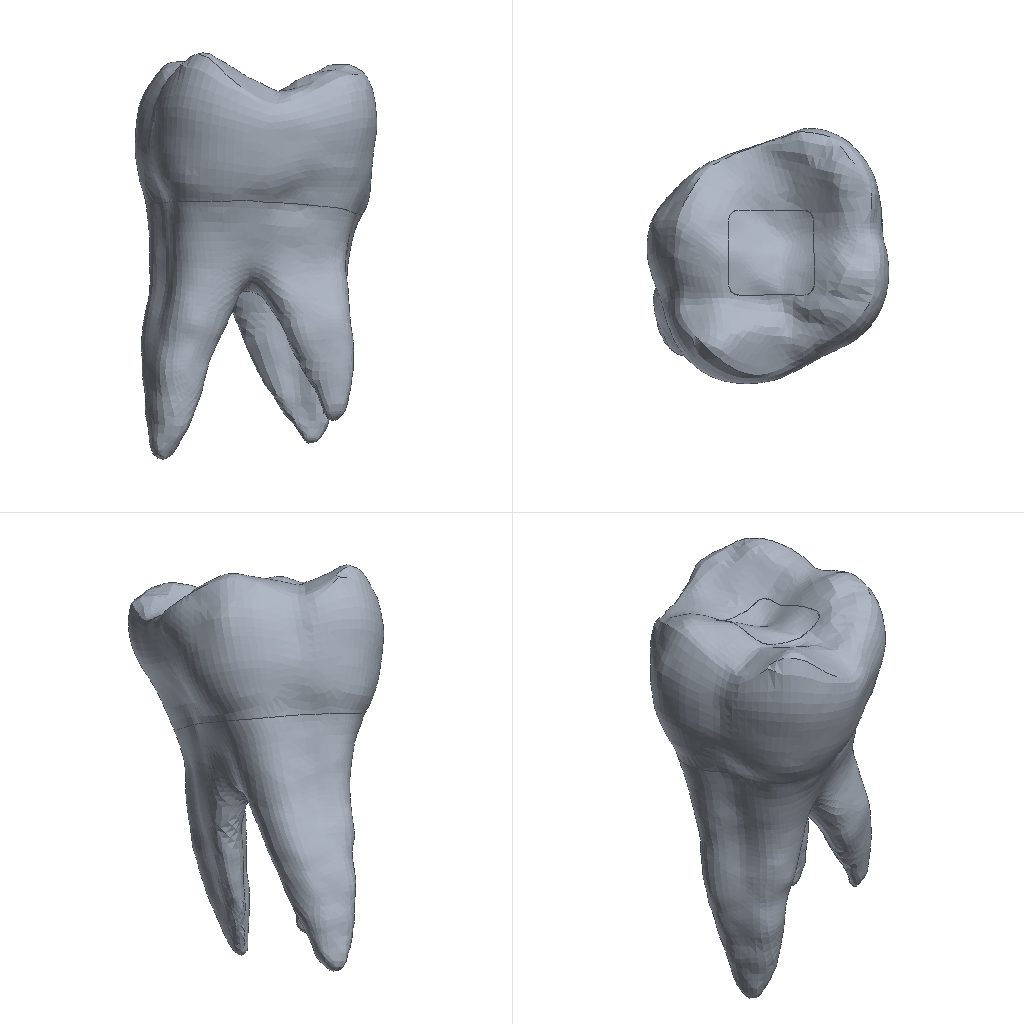Simulation study | abaqus
Set-up summary:
category,name,step,type,value,unit,region
solver,abaqus
solver,version,,,Abaqus/Standard 2020
units,not stated in the deck,,not stated
analysis,deck,,thermal,thermal
load_step,Step-1,Step-1,thermal
load_step,requested,,,1
mesh,nodes,,,60960
mesh,elements,,,308773
element_type,DC3D4,,solid,308773
load,load commands in deck,,count,3
bc,support commands in deck,,count,1
material,DENTIN,,in results
material,ENAMEL,,in results
material,PULP,,in results
material,REIN,,in results
check,setup vs results,,match,"per instance, exact: element labels, types and connectivity; labels of the nodes the elements use; coordinates of those nodes at SINGLE_PRECISION in 4 of 4 instance(s)"
Abaqus input file, long lists of numbers shortened:
*Heading
** Job name: Job-1 Model name: TRY-15
** Generated by: Abaqus/CAE 2020
*Preprint, echo=NO, model=NO, history=NO, contact=NO
**
** PARTS
**
*Part, name=DETIN
*Node
      1,  -35.692,   -2.365,   11.829
      2,    -35.895,  -2.58,   11.818
** (44272 more lines like these left out)
*Element, type=DC3D4
     1, 12572, 12573, 12574, 12575
     2, 12572, 12576, 12577, 12578
** (231746 more lines like these left out)
*Nset, nset=DENTIN, generate
     1,  44274,      1
*Elset, elset=DENTIN, generate
      1,  231748,       1
*Elset, elset=_D-E_S3, internal
     66,    221,    538,    591,   1106,   2340,   3456,   4665,   4825,   4830,   5177,   6829,   6834,   7005,   7707,   8070
   8084,   8158,   8403,  10011,  10111,  10508,  10907,  10925,  12002,  12020,  12028,  12047,  12055,  12064,  12070,  12081
** (190 more lines like these left out)
*Elset, elset=_D-E_S4, internal
   1151,   1255,   1465,   1975,   5425,   6041,   7050,   8616,   8690,  10700,  10803,  11765,  13500,  15389,  15707,  23011
  25378,  25675,  25833,  25975,  26199,  26378,  29076,  29227,  29399,  29698,  30054,  30055,  32651,  33230,  33251,  33540
** (14 more lines like these left out)
*Elset, elset=_D-E_S2, internal
   1416,   1904,   2071,   4147,   5318,   7713,   9028,  10010,  10024,  10486,  12316,  12331,  12948,  13747,  22977,  25703
  25749,  25763,  25879,  25990,  26349,  29128,  29407,  29462,  29466,  29473,  29507,  29584,  29591,  29596,  29602,  29663
** (15 more lines like these left out)
*Elset, elset=_D-E_S1, internal
   5733,  11885,  12062,  12813,  13750,  13996,  14000,  14123,  14282,  14419,  24990,  25641,  25720,  25947,  25990,  26290
  26311,  27827,  29314,  29569,  29677,  29698,  30069,  30103,  32924,  33012,  33024,  33156,  33187,  33225,  33251,  33472
** (14 more lines like these left out)
*Elset, elset=_D-R_S3, internal
   5734,   6686,   6964,   7429,   7457,   9157,  10041,  10109,  10355,  11055,  12136,  12138,  12290,  12337,  12498,  12806
  12815,  12836,  12952,  13340,  13438,  13445,  13514,  13552,  13755,  13855,  13946,  14031,  14061,  14116,  14465,  20872
** (34 more lines like these left out)
*Elset, elset=_D-R_S4, internal
   6450,  25895,  29323,  29359,  30035,  32601,  33024,  36247,  46250,  49133,  97027,  99941, 107238, 112465, 121080, 131481
 133725, 137569, 139854, 142716, 144027, 164053, 170285, 176348, 189297, 221559
*Elset, elset=_D-R_S1, internal
  22984,  25706,  25921,  26205,  29095,  29096,  29821,  32855,  32937,  36596,  38121,  40083,  43461,  85559,  87495,  87596
 103786, 108863, 111221, 111935, 142008, 143946, 149051, 149554, 162747, 167614, 169637, 175206, 179761, 183881, 205859
*Elset, elset=_D-R_S2, internal
   4550,   6181,  11968,  22962,  22985,  23017,  25463,  25798,  25843,  26000,  26085,  26148,  26231,  29060,  29073,  29092
  29104,  29110,  29251,  29725,  29755,  29846,  32441,  32442,  32829,  32854,  32886,  32936,  33212, 138750
*Elset, elset=_D-P_S3, internal
     38,    157,    343,    405,    497,    643,    734,    945,   1441,   1678,   1894,   2442,   2647,   2918,   2976,   3287
   3440,   3483,   3969,   3999,   4509,   4512,   4551,   4620,   4641,   5890,   6421,   6490,   6691,   6812,   7019,   7151
** (652 more lines like these left out)
*Elset, elset=_D-P_S2, internal
    529,    944,    949,   1000,   1007,   1584,   1585,   1731,   4072,   4205,   4418,   5149,   5374,   5549,   6425,   7188
   7376,   7666,   8660,   9682,   9846,   9975,  10014,  10029,  10033,  10837,  10842,  13021,  13267,  13346,  13366,  13528
** (37 more lines like these left out)
*Elset, elset=_D-P_S4, internal
    426,    464,   1062,   1239,   1483,   1662,   2900,   4324,   4745,   4791,   4969,   5155,   5215,   5630,   6037,   6276
   6317,   6334,   6460,   6528,   6608,   6650,   7446,   7587,   7627,   8168,   9240,   9388,   9636,   9662,   9764,   9791
** (58 more lines like these left out)
*Elset, elset=_D-P_S1, internal
   1399,   4556,  12933,  13162,  13300,  13832,  14011,  14304,  14360,  14492,  15342,  16105,  16819,  16854,  17440,  18440
  18786,  18988,  19585,  19938,  19957,  19982,  19987,  21704,  21817,  22118,  22288,  23956,  24055,  24170,  24432,  27384
** (47 more lines like these left out)
*Elset, elset=_D-E_S3_1, internal
     66,    221,    538,    591,   1106,   2340,   3456,   4665,   4825,   4830,   5177,   6829,   6834,   7005,   7707,   8070
   8084,   8158,   8403,  10011,  10111,  10508,  10907,  10925,  12002,  12020,  12028,  12047,  12055,  12064,  12070,  12081
** (190 more lines like these left out)
*Elset, elset=_D-E_S4_1, internal
   1151,   1255,   1465,   1975,   5425,   6041,   7050,   8616,   8690,  10700,  10803,  11765,  13500,  15389,  15707,  23011
  25378,  25675,  25833,  25975,  26199,  26378,  29076,  29227,  29399,  29698,  30054,  30055,  32651,  33230,  33251,  33540
** (14 more lines like these left out)
*Elset, elset=_D-E_S2_1, internal
   1416,   1904,   2071,   4147,   5318,   7713,   9028,  10010,  10024,  10486,  12316,  12331,  12948,  13747,  22977,  25703
  25749,  25763,  25879,  25990,  26349,  29128,  29407,  29462,  29466,  29473,  29507,  29584,  29591,  29596,  29602,  29663
** (15 more lines like these left out)
*Elset, elset=_D-E_S1_1, internal
   5733,  11885,  12062,  12813,  13750,  13996,  14000,  14123,  14282,  14419,  24990,  25641,  25720,  25947,  25990,  26290
  26311,  27827,  29314,  29569,  29677,  29698,  30069,  30103,  32924,  33012,  33024,  33156,  33187,  33225,  33251,  33472
** (14 more lines like these left out)
*Surface, type=ELEMENT, name=D-E
_D-E_S3_1, S3
_D-E_S4_1, S4
_D-E_S2_1, S2
_D-E_S1_1, S1
*Elset, elset=_D-R_S3_1, internal
   5734,   6686,   6964,   7429,   7457,   9157,  10041,  10109,  10355,  11055,  12136,  12138,  12290,  12337,  12498,  12806
  12815,  12836,  12952,  13340,  13438,  13445,  13514,  13552,  13755,  13855,  13946,  14031,  14061,  14116,  14465,  20872
** (34 more lines like these left out)
*Elset, elset=_D-R_S4_1, internal
   6450,  25895,  29323,  29359,  30035,  32601,  33024,  36247,  46250,  49133,  97027,  99941, 107238, 112465, 121080, 131481
 133725, 137569, 139854, 142716, 144027, 164053, 170285, 176348, 189297, 221559
*Elset, elset=_D-R_S2_1, internal
   4550,   6181,  11968,  22962,  22985,  23017,  25463,  25798,  25843,  26000,  26085,  26148,  26231,  29060,  29073,  29092
  29104,  29110,  29251,  29725,  29755,  29846,  32441,  32442,  32829,  32854,  32886,  32936,  33212, 138750
*Elset, elset=_D-R_S1_1, internal
  22984,  25706,  25921,  26205,  29095,  29096,  29821,  32855,  32937,  36596,  38121,  40083,  43461,  85559,  87495,  87596
 103786, 108863, 111221, 111935, 142008, 143946, 149051, 149554, 162747, 167614, 169637, 175206, 179761, 183881, 205859
*Surface, type=ELEMENT, name=D-R
_D-R_S3_1, S3
_D-R_S4_1, S4
_D-R_S2_1, S2
_D-R_S1_1, S1
*Elset, elset=_D-P_S3_1, internal
     38,    157,    343,    405,    497,    643,    734,    945,   1441,   1678,   1894,   2442,   2647,   2918,   2976,   3287
   3440,   3483,   3969,   3999,   4509,   4512,   4551,   4620,   4641,   5890,   6421,   6490,   6691,   6812,   7019,   7151
** (652 more lines like these left out)
*Elset, elset=_D-P_S2_1, internal
    529,    944,    949,   1000,   1007,   1584,   1585,   1731,   4072,   4205,   4418,   5149,   5374,   5549,   6425,   7188
   7376,   7666,   8660,   9682,   9846,   9975,  10014,  10029,  10033,  10837,  10842,  13021,  13267,  13346,  13366,  13528
** (37 more lines like these left out)
*Elset, elset=_D-P_S4_1, internal
    426,    464,   1062,   1239,   1483,   1662,   2900,   4324,   4745,   4791,   4969,   5155,   5215,   5630,   6037,   6276
   6317,   6334,   6460,   6528,   6608,   6650,   7446,   7587,   7627,   8168,   9240,   9388,   9636,   9662,   9764,   9791
** (58 more lines like these left out)
*Elset, elset=_D-P_S1_1, internal
   1399,   4556,  12933,  13162,  13300,  13832,  14011,  14304,  14360,  14492,  15342,  16105,  16819,  16854,  17440,  18440
  18786,  18988,  19585,  19938,  19957,  19982,  19987,  21704,  21817,  22118,  22288,  23956,  24055,  24170,  24432,  27384
** (47 more lines like these left out)
*Surface, type=ELEMENT, name=D-P
_D-P_S3_1, S3
_D-P_S2_1, S2
_D-P_S4_1, S4
_D-P_S1_1, S1
** Section: Section-1-DENTIN
*Solid Section, elset=DENTIN, material=DENTIN
,
*End Part
**
*Part, name=ENAMEL
*Node
      1,  -28.183,   3.777,   29.443
      2,  -28.797,   3.864,   29.053
** (5959 more lines like these left out)
*Element, type=DC3D4
    1, 3366, 3367, 3368, 3114
    2, 3369, 3370, 3371, 3372
** (25664 more lines like these left out)
*Nset, nset=ENAMEL, generate
    1,  5961,     1
*Elset, elset=ENAMEL, generate
     1,  25666,      1
*Elset, elset=_E-D_S1, internal
   115,   143,   670,   914,   964,  1200,  1350,  1379,  1460,  1844,  1861,  2247,  2711,  2858,  2866,  3191
  3271,  3777,  3821,  4171,  4200,  4408,  4537,  4602,  4740,  5040,  5071,  5085,  5183,  5429,  5746,  5921
** (12 more lines like these left out)
*Elset, elset=_E-D_S4, internal
   165,   209,   333,   368,   447,   459,   496,   499,   610,   631,   750,   824,   855,   876,   902,   978
   983,  1041,  1208,  1213,  1267,  1312,  1410,  1616,  1861,  1869,  1872,  1965,  2087,  2269,  2291,  2336
** (16 more lines like these left out)
*Elset, elset=_E-D_S3, internal
   133,   211,   581,   754,  1159,  1191,  1305,  1938,  1941,  2050,  2127,  2135,  2196,  2208,  2236,  2586
  2716,  2832,  3492,  3610,  3621,  3742,  3795,  3878,  3928,  4050,  4080,  4109,  4208,  4216,  4495,  4525
** (89 more lines like these left out)
*Elset, elset=_E-D_S2, internal
    61,   172,   670,   780,   897,  1442,  1460,  1600,  1706,  2070,  2101,  2247,  2253,  2395,  2476,  2721
  3037,  3130,  3158,  3363,  3556,  3563,  3565,  3637,  3774,  3803,  3860,  3862,  3883,  4301,  4388,  4609
** (17 more lines like these left out)
*Elset, elset=_E-R_S3, internal
   430,  1554,  2274,  2276,  2506,  5430,  5565,  5770,  5921,  6035,  6063,  6080,  6089,  6097,  6252,  6328
  6374,  6429,  6546,  6548,  6670,  6739,  6751,  6795,  6825,  6870,  6964,  6976,  6995,  7512,  7556,  7609
** (12 more lines like these left out)
*Elset, elset=_E-R_S1, internal
  5206,  7726,  7980,  8003,  8044,  8060,  9845,  9935,  9946,  9956, 10215, 12186, 12265, 12387, 12397, 12435
 14290, 14363, 15500, 17973
*Elset, elset=_E-R_S2, internal
  5834,  6272,  7742,  7757,  7774,  9650,  9659,  9671,  9732,  9735,  9779,  9885,  9936,  9971, 10125, 10345
 10465, 10496, 12187, 12244, 12251, 12322, 12350, 12384, 12392, 12416, 12427, 12445, 12455, 12459, 12463, 12467
** (1 more lines like these left out)
*Elset, elset=_E-R_S4, internal
  6037,  7704,  7722,  8024,  8089,  9812, 10348, 10462, 11325, 12056, 12348, 12359, 12497, 14007, 15132, 22901
 25238,
*Elset, elset=_E-D_S1_1, internal
   115,   143,   670,   914,   964,  1200,  1350,  1379,  1460,  1844,  1861,  2247,  2711,  2858,  2866,  3191
  3271,  3777,  3821,  4171,  4200,  4408,  4537,  4602,  4740,  5040,  5071,  5085,  5183,  5429,  5746,  5921
** (12 more lines like these left out)
*Elset, elset=_E-D_S4_1, internal
   165,   209,   333,   368,   447,   459,   496,   499,   610,   631,   750,   824,   855,   876,   902,   978
   983,  1041,  1208,  1213,  1267,  1312,  1410,  1616,  1861,  1869,  1872,  1965,  2087,  2269,  2291,  2336
** (16 more lines like these left out)
*Elset, elset=_E-D_S2_1, internal
    61,   172,   670,   780,   897,  1442,  1460,  1600,  1706,  2070,  2101,  2247,  2253,  2395,  2476,  2721
  3037,  3130,  3158,  3363,  3556,  3563,  3565,  3637,  3774,  3803,  3860,  3862,  3883,  4301,  4388,  4609
** (17 more lines like these left out)
*Elset, elset=_E-D_S3_1, internal
   133,   211,   581,   754,  1159,  1191,  1305,  1938,  1941,  2050,  2127,  2135,  2196,  2208,  2236,  2586
  2716,  2832,  3492,  3610,  3621,  3742,  3795,  3878,  3928,  4050,  4080,  4109,  4208,  4216,  4495,  4525
** (89 more lines like these left out)
*Surface, type=ELEMENT, name=E-D
_E-D_S1_1, S1
_E-D_S4_1, S4
_E-D_S2_1, S2
_E-D_S3_1, S3
*Elset, elset=_E-R_S3_1, internal
   430,  1554,  2274,  2276,  2506,  5430,  5565,  5770,  5921,  6035,  6063,  6080,  6089,  6097,  6252,  6328
  6374,  6429,  6546,  6548,  6670,  6739,  6751,  6795,  6825,  6870,  6964,  6976,  6995,  7512,  7556,  7609
** (12 more lines like these left out)
*Elset, elset=_E-R_S1_1, internal
  5206,  7726,  7980,  8003,  8044,  8060,  9845,  9935,  9946,  9956, 10215, 12186, 12265, 12387, 12397, 12435
 14290, 14363, 15500, 17973
*Elset, elset=_E-R_S2_1, internal
  5834,  6272,  7742,  7757,  7774,  9650,  9659,  9671,  9732,  9735,  9779,  9885,  9936,  9971, 10125, 10345
 10465, 10496, 12187, 12244, 12251, 12322, 12350, 12384, 12392, 12416, 12427, 12445, 12455, 12459, 12463, 12467
** (1 more lines like these left out)
*Elset, elset=_E-R_S4_1, internal
  6037,  7704,  7722,  8024,  8089,  9812, 10348, 10462, 11325, 12056, 12348, 12359, 12497, 14007, 15132, 22901
 25238,
*Surface, type=ELEMENT, name=E-R
_E-R_S3_1, S3
_E-R_S1_1, S1
_E-R_S2_1, S2
_E-R_S4_1, S4
** Section: Section-2-ENAMEL
*Solid Section, elset=ENAMEL, material=ENAMEL
,
*End Part
**
*Part, name=PULP
*Node
      1,  -28.856,   1.883,   12.951
      2,  -28.926,   1.922,   13.002
** (2159 more lines like these left out)
*Element, type=DC3D4
   1, 1687, 1688, 1689, 1690
   2, 1496, 1691, 1692, 1693
** (7371 more lines like these left out)
*Nset, nset=PULP, generate
    1,  2161,     1
*Elset, elset=PULP, generate
    1,  7373,     1
*Elset, elset=_P-D_S3, internal
   15,   18,  127,  169,  172,  208,  209,  239,  243,  252,  294,  312,  337,  381,  382,  383
  410,  429,  440,  466,  469,  471,  472,  475,  498,  523,  524,  527,  529,  540,  546,  562
** (136 more lines like these left out)
*Elset, elset=_P-D_S2, internal
  158,  176,  293,  522,  576,  581,  645,  719,  756,  776,  820,  970, 1052, 1095, 1213, 1325
 1356, 1364, 1371, 1374, 1479, 1544, 1710, 1730, 1788, 2008, 2192, 2275, 2336, 2462, 2466, 2493
** (24 more lines like these left out)
*Elset, elset=_P-D_S4, internal
    7,   66,   84,  122,  176,  219,  234,  275,  303,  315,  323,  336,  407,  409,  442,  567
  574,  581,  594,  646,  652,  653,  703,  725,  734,  746,  756,  820,  822,  846,  851,  853
** (23 more lines like these left out)
*Elset, elset=_P-D_S1, internal
   19,  113,  139,  326,  380,  385,  431,  432,  533,  548,  569,  575,  576,  597,  651,  719
  724,  785,  940,  969, 1130, 1152, 1155, 1198, 1205, 1213, 1227, 1267, 1283, 1293, 1309, 1367
** (21 more lines like these left out)
*Elset, elset=_P-D_S3_1, internal
   15,   18,  127,  169,  172,  208,  209,  239,  243,  252,  294,  312,  337,  381,  382,  383
  410,  429,  440,  466,  469,  471,  472,  475,  498,  523,  524,  527,  529,  540,  546,  562
** (136 more lines like these left out)
*Elset, elset=_P-D_S2_1, internal
  158,  176,  293,  522,  576,  581,  645,  719,  756,  776,  820,  970, 1052, 1095, 1213, 1325
 1356, 1364, 1371, 1374, 1479, 1544, 1710, 1730, 1788, 2008, 2192, 2275, 2336, 2462, 2466, 2493
** (24 more lines like these left out)
*Elset, elset=_P-D_S4_1, internal
    7,   66,   84,  122,  176,  219,  234,  275,  303,  315,  323,  336,  407,  409,  442,  567
  574,  581,  594,  646,  652,  653,  703,  725,  734,  746,  756,  820,  822,  846,  851,  853
** (23 more lines like these left out)
*Elset, elset=_P-D_S1_1, internal
   19,  113,  139,  326,  380,  385,  431,  432,  533,  548,  569,  575,  576,  597,  651,  719
  724,  785,  940,  969, 1130, 1152, 1155, 1198, 1205, 1213, 1227, 1267, 1283, 1293, 1309, 1367
** (21 more lines like these left out)
*Surface, type=ELEMENT, name=P-D
_P-D_S3_1, S3
_P-D_S2_1, S2
_P-D_S4_1, S4
_P-D_S1_1, S1
** Section: Section-3-PULP
*Solid Section, elset=PULP, material=PULP
,
*End Part
**
*Part, name=RESIN
*Node
      1,  -32.961,  0.757,   29.601
      2,  -32.366, -0.09989,   29.248
** (8562 more lines like these left out)
*Element, type=DC3D4
    1, 2430, 2431, 2432, 2433
    2, 2433, 2434, 2435, 2436
** (43984 more lines like these left out)
*Nset, nset=RESIN, generate
    1,  8564,     1
*Elset, elset=RESIN, generate
     1,  43986,      1
*Elset, elset=_R_S3, internal
    24,   113,   201,   244,   248,   295,   312,   333,   340,   358,   388,   416,   442,   507,   531,   616
   719,   889,   896,   930,   939,   968,   983,  1047,  1064,  1073,  1144,  1160,  1162,  1164,  1166,  1167
** (225 more lines like these left out)
*Elset, elset=_R_S4, internal
    28,    36,   124,  2532,  4101,  4446,  4624,  4978,  5103,  5249,  5369,  5587,  5678,  5836,  5892,  5976
  5991,  6000,  6002,  6025,  6134,  6337,  6533,  6635,  6686,  7400,  7426,  7481,  7482,  7540,  7625,  7720
** (6 more lines like these left out)
*Elset, elset=_R_S2, internal
   149,   415,  2198,  2391,  2787,  2852,  3177,  3279,  4046,  4425,  4964,  4981,  4997,  5010,  5057,  5104
  5155,  5186,  5721,  5964,  6220,  6354,  6754,  6886,  6916,  6920,  6953,  6995,  7277,  7355,  7357,  7404
** (5 more lines like these left out)
*Elset, elset=_R_S1, internal
  1737,  2297,  2467,  2862,  4487,  4612,  5029,  5099,  5350,  5925,  6310,  6317,  7417,  7566,  7622,  7681
  7784,  7785,  7788,  7958,  9654, 10792, 12184, 12298, 12511, 12536, 12881, 13228, 13867, 14506, 15041, 15430
** (4 more lines like these left out)
*Elset, elset=_R_S3_1, internal
    24,   113,   201,   244,   248,   295,   312,   333,   340,   358,   388,   416,   442,   507,   531,   616
   719,   889,   896,   930,   939,   968,   983,  1047,  1064,  1073,  1144,  1160,  1162,  1164,  1166,  1167
** (225 more lines like these left out)
*Elset, elset=_R_S4_1, internal
    28,    36,   124,  2532,  4101,  4446,  4624,  4978,  5103,  5249,  5369,  5587,  5678,  5836,  5892,  5976
  5991,  6000,  6002,  6025,  6134,  6337,  6533,  6635,  6686,  7400,  7426,  7481,  7482,  7540,  7625,  7720
** (6 more lines like these left out)
*Elset, elset=_R_S2_1, internal
   149,   415,  2198,  2391,  2787,  2852,  3177,  3279,  4046,  4425,  4964,  4981,  4997,  5010,  5057,  5104
  5155,  5186,  5721,  5964,  6220,  6354,  6754,  6886,  6916,  6920,  6953,  6995,  7277,  7355,  7357,  7404
** (5 more lines like these left out)
*Elset, elset=_R_S1_1, internal
  1737,  2297,  2467,  2862,  4487,  4612,  5029,  5099,  5350,  5925,  6310,  6317,  7417,  7566,  7622,  7681
  7784,  7785,  7788,  7958,  9654, 10792, 12184, 12298, 12511, 12536, 12881, 13228, 13867, 14506, 15041, 15430
** (4 more lines like these left out)
*Surface, type=ELEMENT, name=R
_R_S3_1, S3
_R_S4_1, S4
_R_S2_1, S2
_R_S1_1, S1
** Section: Section-4-RESIN
*Solid Section, elset=RESIN, material=REIN
,
*End Part
**
**
** ASSEMBLY
**
*Assembly, name=Assembly
**
*Instance, name=DETIN-1, part=DETIN
*End Instance
**
*Instance, name=ENAMEL-1, part=ENAMEL
*End Instance
**
*Instance, name=PULP-1, part=PULP
*End Instance
**
*Instance, name=RESIN-1, part=RESIN
*End Instance
**
*Nset, nset=SET-1, instance=DETIN-1, generate
     1,  44274,      1
*Nset, nset=SET-1, instance=RESIN-1, generate
    1,  8564,     1
*Nset, nset=SET-1, instance=PULP-1, generate
    1,  2161,     1
*Nset, nset=SET-1, instance=ENAMEL-1, generate
    1,  5961,     1
*Elset, elset=SET-1, instance=DETIN-1, generate
      1,  231748,       1
*Elset, elset=SET-1, instance=RESIN-1, generate
     1,  43986,      1
*Elset, elset=SET-1, instance=PULP-1, generate
    1,  7373,     1
*Elset, elset=SET-1, instance=ENAMEL-1, generate
     1,  25666,      1
*Nset, nset=SET-2, instance=DETIN-1
     1,     2,     3,     4,     5,     6,     7,     8,     9,    10,    11,    12,    13,    14,    15,    16
    17,    18,    19,    20,    21,    22,    23,    24,    25,    26,    27,    28,    29,    30,    31,    32
** (248 more lines like these left out)
*Nset, nset=SET-2, instance=RESIN-1
    1,    2,    3,    4,    8,    9,   10,   11,   12,   13,   14,   15,   16,   17,   18,   19
   20,   21,   22,   23,   26,   27,   28,   29,   32,   33,   34,   35,   36,   37,   38,   39
** (30 more lines like these left out)
*Nset, nset=SET-2, instance=ENAMEL-1
    1,    2,    3,    4,    5,    6,    7,    8,    9,   10,   11,   12,   13,   14,   15,   16
   17,   18,   19,   20,   21,   22,   23,   24,   25,   26,   27,   28,   29,   30,   31,   32
** (133 more lines like these left out)
*Elset, elset=SET-2, instance=DETIN-1
     39,     63,    202,    319,    323,    371,    627,    717,    892,   1188,   1326,   1374,   1498,   1648,   2102,   2213
   2552,   2850,   2864,   2878,   3139,   3482,   3491,   3813,   4136,   4261,   4599,   4923,   5022,   5173,   5808,   6070
** (490 more lines like these left out)
*Elset, elset=SET-2, instance=RESIN-1
   177,   198,  1086,  1100,  1258,  1321,  1601,  1683,  1737,  1931,  1971,  2040,  2135,  2145,  2216,  2467
  2529,  2832,  2852,  2862,  2955,  3045,  3068,  3252,  3306,  3398,  3407,  3824,  3825,  3845,  3862,  3875
** (57 more lines like these left out)
*Elset, elset=SET-2, instance=ENAMEL-1
   115,   185,   348,   408,   411,   590,   614,   616,   645,   811,   828,   850,   852,   988,  1005,  1068
  1090,  1129,  1149,  1152,  1197,  1199,  1360,  1376,  1379,  1431,  1462,  1475,  1508,  1514,  1517,  1520
** (260 more lines like these left out)
*Nset, nset=SET-3, instance=ENAMEL-1
    1,    2,    3,    4,    5,    6,    7,    8,    9,   10,   11,   12,   13,   14,   15,   16
   17,   18,   19,   20,   21,   22,   23,   24,   25,   26,   27,   28,   29,   30,   31,   32
** (133 more lines like these left out)
*Nset, nset=SET-3, instance=RESIN-1
    1,    2,    3,    4,    8,    9,   10,   11,   12,   13,   14,   15,   16,   17,   18,   19
   20,   21,   22,   23,   26,   27,   28,   29,   32,   33,   34,   35,   36,   37,   38,   39
** (30 more lines like these left out)
*Elset, elset=SET-3, instance=ENAMEL-1
   115,   185,   348,   408,   411,   590,   614,   616,   645,   811,   828,   850,   852,   988,  1005,  1068
  1090,  1129,  1149,  1152,  1197,  1199,  1360,  1376,  1379,  1431,  1462,  1475,  1508,  1514,  1517,  1520
** (260 more lines like these left out)
*Elset, elset=SET-3, instance=RESIN-1
   177,   198,  1086,  1100,  1258,  1321,  1601,  1683,  1737,  1931,  1971,  2040,  2135,  2145,  2216,  2467
  2529,  2832,  2852,  2862,  2955,  3045,  3068,  3252,  3306,  3398,  3407,  3824,  3825,  3845,  3862,  3875
** (57 more lines like these left out)
*Elset, elset=_Surf-1_S1, internal, instance=DETIN-1
    323,   1399,   4556,   5733,  11645,  11885,  12062,  12331,  12813,  12933,  13029,  13162,  13240,  13265,  13300,  13750
  13819,  13832,  13977,  13996,  14000,  14011,  14123,  14282,  14304,  14360,  14419,  14492,  14561,  14735,  14875,  14892
** (83 more lines like these left out)
*Elset, elset=_Surf-1_S1, internal, instance=ENAMEL-1
   115,   143,   645,   670,   914,   964,  1200,  1350,  1379,  1460,  1517,  1576,  1844,  1861,  1870,  1964
  2247,  2314,  2333,  2711,  2858,  2866,  3191,  3271,  3310,  3652,  3777,  3821,  4171,  4200,  4228,  4301
** (30 more lines like these left out)
*Elset, elset=_Surf-1_S1, internal, instance=PULP-1
   19,  113,  139,  326,  380,  385,  431,  432,  533,  548,  569,  575,  576,  597,  651,  719
  724,  785,  940,  969, 1130, 1152, 1155, 1198, 1205, 1213, 1227, 1267, 1283, 1293, 1309, 1367
** (21 more lines like these left out)
*Elset, elset=_Surf-1_S1, internal, instance=RESIN-1
  1737,  2297,  2467,  2862,  4487,  4612,  5029,  5099,  5137,  5350,  5821,  5925,  6310,  6317,  6354,  6390
  7417,  7566,  7622,  7681,  7784,  7785,  7788,  7958,  9654, 10792, 11150, 12184, 12269, 12298, 12511, 12536
** (5 more lines like these left out)
*Elset, elset=_Surf-1_S2, internal, instance=DETIN-1
    529,    627,    717,    944,    949,   1000,   1007,   1374,   1416,   1584,   1585,   1648,   1731,   1904,   2071,   2864
   4072,   4147,   4205,   4418,   4550,   5149,   5318,   5374,   5549,   5808,   6181,   6425,   6776,   6779,   6787,   7188
** (76 more lines like these left out)
*Elset, elset=_Surf-1_S2, internal, instance=ENAMEL-1
    61,   115,   172,   670,   780,   811,   897,  1379,  1442,  1460,  1475,  1520,  1525,  1600,  1685,  1706
  1757,  2070,  2101,  2247,  2253,  2395,  2435,  2476,  2564,  2694,  2721,  3037,  3130,  3158,  3210,  3319
** (42 more lines like these left out)
*Elset, elset=_Surf-1_S2, internal, instance=PULP-1
  158,  176,  293,  522,  576,  581,  645,  719,  756,  776,  820,  970, 1052, 1095, 1213, 1325
 1356, 1364, 1371, 1374, 1479, 1544, 1710, 1730, 1788, 2008, 2192, 2275, 2336, 2462, 2466, 2493
** (24 more lines like these left out)
*Elset, elset=_Surf-1_S2, internal, instance=RESIN-1
   149,   415,  1931,  2198,  2391,  2787,  2852,  2955,  3177,  3279,  3845,  3921,  4046,  4221,  4425,  4964
  4981,  4997,  5010,  5057,  5104,  5131,  5147,  5155,  5186,  5721,  5791,  5836,  5844,  5964,  6220,  6354
** (7 more lines like these left out)
*Elset, elset=_Surf-1_S3, internal, instance=DETIN-1
     38,     39,     63,     66,    157,    202,    221,    319,    343,    405,    497,    538,    591,    643,    734,    892
    945,   1106,   1188,   1441,   1498,   1678,   1894,   2102,   2213,   2340,   2442,   2552,   2647,   2850,   2878,   2918
** (1306 more lines like these left out)
*Elset, elset=_Surf-1_S3, internal, instance=ENAMEL-1
   133,   185,   211,   348,   408,   430,   581,   590,   616,   754,   828,   850,   988,  1005,  1090,  1129
  1149,  1152,  1159,  1191,  1199,  1305,  1360,  1376,  1514,  1554,  1702,  1771,  1845,  1938,  1941,  1946
** (305 more lines like these left out)
*Elset, elset=_Surf-1_S3, internal, instance=PULP-1
   15,   18,  127,  169,  172,  208,  209,  239,  243,  252,  294,  312,  337,  381,  382,  383
  410,  429,  440,  466,  469,  471,  472,  475,  498,  523,  524,  527,  529,  540,  546,  562
** (136 more lines like these left out)
*Elset, elset=_Surf-1_S3, internal, instance=RESIN-1
    24,   113,   201,   244,   248,   295,   312,   333,   340,   358,   388,   416,   442,   507,   531,   616
   719,   889,   896,   930,   939,   968,   983,  1047,  1064,  1073,  1086,  1100,  1144,  1160,  1162,  1164
** (277 more lines like these left out)
*Elset, elset=_Surf-1_S4, internal, instance=DETIN-1
    371,    426,    464,   1062,   1151,   1239,   1255,   1326,   1465,   1483,   1662,   1975,   2900,   4324,   4745,   4791
   4969,   5155,   5215,   5425,   5630,   6037,   6041,   6070,   6088,   6276,   6317,   6334,   6382,   6450,   6460,   6528
** (100 more lines like these left out)
*Elset, elset=_Surf-1_S4, internal, instance=ENAMEL-1
   165,   209,   333,   368,   411,   447,   459,   496,   499,   610,   614,   631,   750,   824,   852,   855
   876,   902,   978,   983,  1041,  1068,  1197,  1208,  1213,  1267,  1312,  1410,  1431,  1462,  1508,  1616
** (38 more lines like these left out)
*Elset, elset=_Surf-1_S4, internal, instance=PULP-1
    7,   66,   84,  122,  176,  219,  234,  275,  303,  315,  323,  336,  407,  409,  442,  567
  574,  581,  594,  646,  652,  653,  703,  725,  734,  746,  756,  820,  822,  846,  851,  853
** (23 more lines like these left out)
*Elset, elset=_Surf-1_S4, internal, instance=RESIN-1
    28,    36,   124,   177,   198,  1321,  2532,  4101,  4169,  4446,  4624,  4884,  4928,  4978,  5103,  5249
  5369,  5587,  5678,  5773,  5804,  5836,  5858,  5892,  5976,  5991,  6000,  6002,  6025,  6134,  6337,  6437
** (8 more lines like these left out)
*Surface, type=ELEMENT, name=Surf-1
_Surf-1_S1, S1
_Surf-1_S2, S2
_Surf-1_S4, S4
_Surf-1_S3, S3
*Elset, elset=_Surf-2_S1, internal, instance=DETIN-1
    323,   1399,   4556,   5733,  11645,  11885,  12062,  12331,  12813,  12933,  13029,  13162,  13240,  13265,  13300,  13750
  13819,  13832,  13977,  13996,  14000,  14011,  14123,  14282,  14304,  14360,  14419,  14492,  14561,  14735,  14875,  14892
** (83 more lines like these left out)
*Elset, elset=_Surf-2_S1, internal, instance=ENAMEL-1
   115,   143,   645,   670,   914,   964,  1200,  1350,  1379,  1460,  1517,  1576,  1844,  1861,  1870,  1964
  2247,  2314,  2333,  2711,  2858,  2866,  3191,  3271,  3310,  3652,  3777,  3821,  4171,  4200,  4228,  4301
** (30 more lines like these left out)
*Elset, elset=_Surf-2_S1, internal, instance=PULP-1
   19,  113,  139,  326,  380,  385,  431,  432,  533,  548,  569,  575,  576,  597,  651,  719
  724,  785,  940,  969, 1130, 1152, 1155, 1198, 1205, 1213, 1227, 1267, 1283, 1293, 1309, 1367
** (21 more lines like these left out)
*Elset, elset=_Surf-2_S1, internal, instance=RESIN-1
  1737,  2297,  2467,  2862,  4487,  4612,  5029,  5099,  5137,  5350,  5821,  5925,  6310,  6317,  6354,  6390
  7417,  7566,  7622,  7681,  7784,  7785,  7788,  7958,  9654, 10792, 11150, 12184, 12269, 12298, 12511, 12536
** (5 more lines like these left out)
*Elset, elset=_Surf-2_S2, internal, instance=DETIN-1
    529,    627,    717,    944,    949,   1000,   1007,   1374,   1416,   1584,   1585,   1648,   1731,   1904,   2071,   2864
   4072,   4147,   4205,   4418,   4550,   5149,   5318,   5374,   5549,   5808,   6181,   6425,   6776,   6779,   6787,   7188
** (76 more lines like these left out)
*Elset, elset=_Surf-2_S2, internal, instance=ENAMEL-1
    61,   115,   172,   670,   780,   811,   897,  1379,  1442,  1460,  1475,  1520,  1525,  1600,  1685,  1706
  1757,  2070,  2101,  2247,  2253,  2395,  2435,  2476,  2564,  2694,  2721,  3037,  3130,  3158,  3210,  3319
** (42 more lines like these left out)
*Elset, elset=_Surf-2_S2, internal, instance=PULP-1
  158,  176,  293,  522,  576,  581,  645,  719,  756,  776,  820,  970, 1052, 1095, 1213, 1325
 1356, 1364, 1371, 1374, 1479, 1544, 1710, 1730, 1788, 2008, 2192, 2275, 2336, 2462, 2466, 2493
** (24 more lines like these left out)
*Elset, elset=_Surf-2_S2, internal, instance=RESIN-1
   149,   415,  1931,  2198,  2391,  2787,  2852,  2955,  3177,  3279,  3845,  3921,  4046,  4221,  4425,  4964
  4981,  4997,  5010,  5057,  5104,  5131,  5147,  5155,  5186,  5721,  5791,  5836,  5844,  5964,  6220,  6354
** (7 more lines like these left out)
*Elset, elset=_Surf-2_S3, internal, instance=DETIN-1
     38,     39,     63,     66,    157,    202,    221,    319,    343,    405,    497,    538,    591,    643,    734,    892
    945,   1106,   1188,   1441,   1498,   1678,   1894,   2102,   2213,   2340,   2442,   2552,   2647,   2850,   2878,   2918
** (1306 more lines like these left out)
*Elset, elset=_Surf-2_S3, internal, instance=ENAMEL-1
   133,   185,   211,   348,   408,   430,   581,   590,   616,   754,   828,   850,   988,  1005,  1090,  1129
  1149,  1152,  1159,  1191,  1199,  1305,  1360,  1376,  1514,  1554,  1702,  1771,  1845,  1938,  1941,  1946
** (305 more lines like these left out)
*Elset, elset=_Surf-2_S3, internal, instance=PULP-1
   15,   18,  127,  169,  172,  208,  209,  239,  243,  252,  294,  312,  337,  381,  382,  383
  410,  429,  440,  466,  469,  471,  472,  475,  498,  523,  524,  527,  529,  540,  546,  562
** (136 more lines like these left out)
*Elset, elset=_Surf-2_S3, internal, instance=RESIN-1
    24,   113,   201,   244,   248,   295,   312,   333,   340,   358,   388,   416,   442,   507,   531,   616
   719,   889,   896,   930,   939,   968,   983,  1047,  1064,  1073,  1086,  1100,  1144,  1160,  1162,  1164
** (277 more lines like these left out)
*Elset, elset=_Surf-2_S4, internal, instance=DETIN-1
    371,    426,    464,   1062,   1151,   1239,   1255,   1326,   1465,   1483,   1662,   1975,   2900,   4324,   4745,   4791
   4969,   5155,   5215,   5425,   5630,   6037,   6041,   6070,   6088,   6276,   6317,   6334,   6382,   6450,   6460,   6528
** (100 more lines like these left out)
*Elset, elset=_Surf-2_S4, internal, instance=ENAMEL-1
   165,   209,   333,   368,   411,   447,   459,   496,   499,   610,   614,   631,   750,   824,   852,   855
   876,   902,   978,   983,  1041,  1068,  1197,  1208,  1213,  1267,  1312,  1410,  1431,  1462,  1508,  1616
** (38 more lines like these left out)
*Elset, elset=_Surf-2_S4, internal, instance=PULP-1
    7,   66,   84,  122,  176,  219,  234,  275,  303,  315,  323,  336,  407,  409,  442,  567
  574,  581,  594,  646,  652,  653,  703,  725,  734,  746,  756,  820,  822,  846,  851,  853
** (23 more lines like these left out)
*Elset, elset=_Surf-2_S4, internal, instance=RESIN-1
    28,    36,   124,   177,   198,  1321,  2532,  4101,  4169,  4446,  4624,  4884,  4928,  4978,  5103,  5249
  5369,  5587,  5678,  5773,  5804,  5836,  5858,  5892,  5976,  5991,  6000,  6002,  6025,  6134,  6337,  6437
** (8 more lines like these left out)
*Surface, type=ELEMENT, name=Surf-2
_Surf-2_S1, S1
_Surf-2_S2, S2
_Surf-2_S4, S4
_Surf-2_S3, S3
** Constraint: D-P-1
*Tie, name=D-P-1, adjust=no, type=SURFACE TO SURFACE
PULP-1.P-D, DETIN-1.D-P
** Constraint: D-R-1
*Tie, name=D-R-1, adjust=no, type=SURFACE TO SURFACE
RESIN-1.R, DETIN-1.D-R
** Constraint: DE-1
*Tie, name=DE-1, adjust=no, type=SURFACE TO SURFACE
ENAMEL-1.E-D, DETIN-1.D-E
** Constraint: E-R-1
*Tie, name=E-R-1, adjust=no, type=SURFACE TO SURFACE
RESIN-1.R, ENAMEL-1.E-R
*End Assembly
**
** MATERIALS
**
*Material, name=DENTIN
*Conductivity
 0.63,
*Density
 2e-09,
*Specific Heat
 1.17e+09,
*Material, name=ENAMEL
*Conductivity
 0.92,
*Density
 2.8e-09,
*Specific Heat
 7.5e+08,
*Material, name=PULP
*Conductivity
 0.67,
*Density
 1e-09,
*Specific Heat
 1e+09,
*Material, name=REIN
*Conductivity
 0.11,
*Density
 2e-09,
*Specific Heat
 8.2e+08,
**
** PHYSICAL CONSTANTS
**
*Physical Constants, absolute zero=-273., stefan boltzmann=5.67e-08
**
** PREDEFINED FIELDS
**
** Name: Field-1   Type: Temperature
*Initial Conditions, type=TEMPERATURE
SET-1, 25.
** ----------------------------------------------------------------
**
** STEP: Step-1
**
*Step, name=Step-1, nlgeom=NO, inc=1000000
*Heat Transfer, steady state, deltmx=1., mxdem=1.
0.01, 30., 0.0003, 30.,
**
** BOUNDARY CONDITIONS
**
** Name: Temp-BC-1 Type: 温度
*Boundary
SET-2, 11, 11, 55.
**
** INTERACTIONS
**
** Interaction: Int-1
*Sradiate
Surf-1, R, 25., 0.5
** Interaction: Int-2
*Sfilm
Surf-2, F, 25., 0.05
**
** OUTPUT REQUESTS
**
*Restart, write, frequency=0
**
** FIELD OUTPUT: F-Output-3
**
*Output, field
*Node Output
NT, RFL
*Element Output, directions=YES
HFL, TEMP
**
** FIELD OUTPUT: F-Output-1
**
*Node Output, nset=RESIN-1.RESIN
NT,
**
** FIELD OUTPUT: F-Output-2
**
*Element Output, elset=RESIN-1.RESIN, directions=YES
TEMP,
**
** HISTORY OUTPUT: H-Output-1
**
*Output, history
*Node Output, nset=RESIN-1.RESIN
NT,
**
** HISTORY OUTPUT: H-Output-2
**
*Element Output, elset=RESIN-1.RESIN
TEMP,
*End Step
Results summary:
result,step,,partial,increments=0 time=0.0/30.0
result,analysis,,,"heat transfer, steady state"
result,last_loadstep,,,1
result,primary field,,,NT11